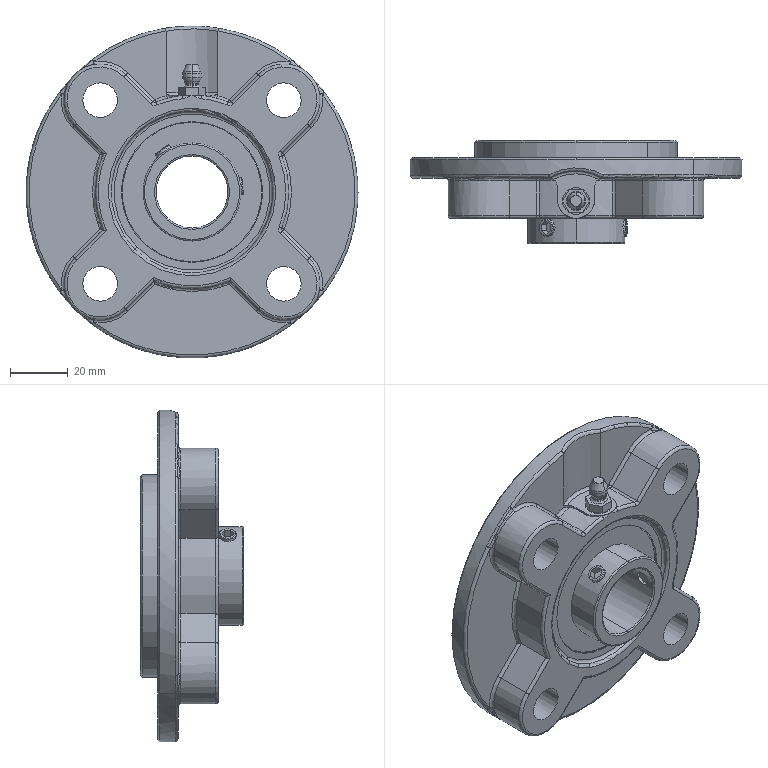Part | STEP file | ucfc_2051V11 | 1 solid | 270 faces | box 115 x 35.698 x 115 mm | volume 136094 mm3 | cylinder 80 | torus 62 | plane 61 | spline 27 | sphere 20 | cone 16 | other 4 | commonest cylinder face diameters 2 x24 12 x8 25 x7 4.917 x6 6 x6 34 x6